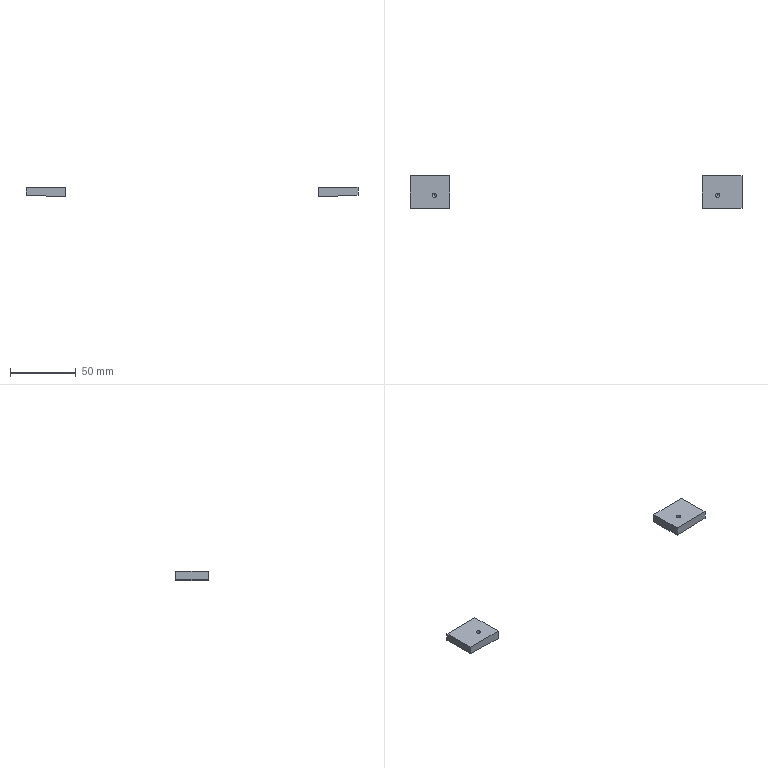Part | STEP file | 526D3-DK_AF1.stp.STEP | 2 solids | 20 faces | box 252 x 25 x 6.851 mm | volume 9576 mm3 | plane 10 | cylinder 6 | cone 4 | commonest cylinder face diameters 3.3 x4 7830 x2
STEP:
#1=CARTESIAN_POINT('',(-107.5,-0.85,-5.));
#2=VERTEX_POINT('',#1);
#3=CARTESIAN_POINT('',(-107.5,-0.85,0.));
#4=VERTEX_POINT('',#3);
#5=CARTESIAN_POINT('',(-107.5,-0.85,-5.));
#6=DIRECTION('',(0.,0.,1.));
#7=VECTOR('',#6,1000.);
#8=LINE('',#5,#7);
#9=EDGE_CURVE('',#2,#4,#8,.T.);
#10=ORIENTED_EDGE('',*,*,#9,.F.);
#11=CARTESIAN_POINT('',(-107.5,-4.15,-5.));
#12=VERTEX_POINT('',#11);
#13=CARTESIAN_POINT('',(-107.5,-2.5,-5.));
#14=DIRECTION('',(0.,0.,-1.));
#15=DIRECTION('',(0.,1.,0.));
#16=AXIS2_PLACEMENT_3D('',#13,#14,#15);
#17=CIRCLE('',#16,1.65);
#18=EDGE_CURVE('',#2,#12,#17,.T.);
#19=ORIENTED_EDGE('',*,*,#18,.T.);
#20=CARTESIAN_POINT('',(-107.5,-4.15,0.));
#21=VERTEX_POINT('',#20);
#22=CARTESIAN_POINT('',(-107.5,-4.15,-5.));
#23=DIRECTION('',(0.,0.,1.));
#24=VECTOR('',#23,1000.);
#25=LINE('',#22,#24);
#26=EDGE_CURVE('',#12,#21,#25,.T.);
#27=ORIENTED_EDGE('',*,*,#26,.T.);
#28=CARTESIAN_POINT('',(-107.5,-2.5,0.));
#29=DIRECTION('',(0.,0.,1.));
#30=DIRECTION('',(0.,-1.,0.));
#31=AXIS2_PLACEMENT_3D('',#28,#29,#30);
#32=CIRCLE('',#31,1.65);
#33=EDGE_CURVE('',#21,#4,#32,.T.);
#34=ORIENTED_EDGE('',*,*,#33,.T.);
#35=EDGE_LOOP('',(#10,#19,#27,#34));
#36=FACE_OUTER_BOUND('',#35,.T.);
#37=CARTESIAN_POINT('',(-107.5,-2.5,-6.291));
#38=DIRECTION('',(0.,0.,1.));
#39=DIRECTION('',(0.,1.,0.));
#40=AXIS2_PLACEMENT_3D('',#37,#38,#39);
#41=CYLINDRICAL_SURFACE('',#40,1.65);
#42=ADVANCED_FACE('',(#36),#41,.F.);
#43=ORIENTED_EDGE('',*,*,#33,.F.);
#44=CARTESIAN_POINT('',(-107.5,-2.5,0.));
#45=DIRECTION('',(0.,0.,1.));
#46=DIRECTION('',(0.,1.,0.));
#47=AXIS2_PLACEMENT_3D('',#44,#45,#46);
#48=CIRCLE('',#47,1.65);
#49=EDGE_CURVE('',#4,#21,#48,.T.);
#50=ORIENTED_EDGE('',*,*,#49,.F.);
#51=EDGE_LOOP('',(#43,#50));
#52=FACE_BOUND('',#51,.T.);
#53=CARTESIAN_POINT('',(-126.,12.5,0.));
#54=VERTEX_POINT('',#53);
#55=CARTESIAN_POINT('',(-96.,12.5,0.));
#56=VERTEX_POINT('',#55);
#57=CARTESIAN_POINT('',(-126.,12.5,0.));
#58=DIRECTION('',(1.,0.,0.));
#59=VECTOR('',#58,1000.);
#60=LINE('',#57,#59);
#61=EDGE_CURVE('',#54,#56,#60,.T.);
#62=ORIENTED_EDGE('',*,*,#61,.F.);
#63=CARTESIAN_POINT('',(-126.,-12.5,0.));
#64=VERTEX_POINT('',#63);
#65=CARTESIAN_POINT('',(-126.,-12.5,0.));
#66=DIRECTION('',(0.,1.,0.));
#67=VECTOR('',#66,1000.);
#68=LINE('',#65,#67);
#69=EDGE_CURVE('',#64,#54,#68,.T.);
#70=ORIENTED_EDGE('',*,*,#69,.F.);
#71=CARTESIAN_POINT('',(-96.,-12.5,0.));
#72=VERTEX_POINT('',#71);
#73=CARTESIAN_POINT('',(-126.,-12.5,0.));
#74=DIRECTION('',(1.,0.,0.));
#75=VECTOR('',#74,1000.);
#76=LINE('',#73,#75);
#77=EDGE_CURVE('',#64,#72,#76,.T.);
#78=ORIENTED_EDGE('',*,*,#77,.T.);
#79=CARTESIAN_POINT('',(-96.,-12.5,0.));
#80=DIRECTION('',(0.,1.,0.));
#81=VECTOR('',#80,1000.);
#82=LINE('',#79,#81);
#83=EDGE_CURVE('',#72,#56,#82,.T.);
#84=ORIENTED_EDGE('',*,*,#83,.T.);
#85=EDGE_LOOP('',(#62,#70,#78,#84));
#86=FACE_OUTER_BOUND('',#85,.T.);
#87=CARTESIAN_POINT('',(-126.,-12.5,0.));
#88=DIRECTION('',(0.,0.,1.));
#89=DIRECTION('',(1.,0.,0.));
#90=AXIS2_PLACEMENT_3D('',#87,#88,#89);
#91=PLANE('',#90);
#92=ADVANCED_FACE('',(#52,#86),#91,.T.);
#93=CARTESIAN_POINT('',(-96.,-12.5,-6.851));
#94=VERTEX_POINT('',#93);
#95=CARTESIAN_POINT('',(-96.,12.5,-6.851));
#96=VERTEX_POINT('',#95);
#97=CARTESIAN_POINT('',(-96.,-12.5,-6.851));
#98=DIRECTION('',(0.,1.,0.));
#99=VECTOR('',#98,1000.);
#100=LINE('',#97,#99);
#101=EDGE_CURVE('',#94,#96,#100,.T.);
#102=ORIENTED_EDGE('',*,*,#101,.T.);
#103=CARTESIAN_POINT('',(-96.,12.5,0.));
#104=DIRECTION('',(0.,0.,-1.));
#105=VECTOR('',#104,1000.);
#106=LINE('',#103,#105);
#107=EDGE_CURVE('',#56,#96,#106,.T.);
#108=ORIENTED_EDGE('',*,*,#107,.F.);
#109=ORIENTED_EDGE('',*,*,#83,.F.);
#110=CARTESIAN_POINT('',(-96.,-12.5,0.));
#111=DIRECTION('',(0.,0.,-1.));
#112=VECTOR('',#111,1000.);
#113=LINE('',#110,#112);
#114=EDGE_CURVE('',#72,#94,#113,.T.);
#115=ORIENTED_EDGE('',*,*,#114,.T.);
#116=EDGE_LOOP('',(#102,#108,#109,#115));
#117=FACE_OUTER_BOUND('',#116,.T.);
#118=CARTESIAN_POINT('',(-96.,12.5,-71.747));
#119=DIRECTION('',(-1.,0.,0.));
#120=DIRECTION('',(0.,0.,1.));
#121=AXIS2_PLACEMENT_3D('',#118,#119,#120);
#122=PLANE('',#121);
#123=ADVANCED_FACE('',(#117),#122,.F.);
#124=ORIENTED_EDGE('',*,*,#77,.F.);
#125=CARTESIAN_POINT('',(-126.,-12.5,-6.));
#126=VERTEX_POINT('',#125);
#127=CARTESIAN_POINT('',(-126.,-12.5,-6.));
#128=DIRECTION('',(0.,0.,1.));
#129=VECTOR('',#128,1000.);
#130=LINE('',#127,#129);
#131=EDGE_CURVE('',#126,#64,#130,.T.);
#132=ORIENTED_EDGE('',*,*,#131,.F.);
#133=CARTESIAN_POINT('',(0.,-12.5,3906.772));
#134=DIRECTION('',(0.,1.,0.));
#135=DIRECTION('',(-0.02452,0.,-0.9997));
#136=AXIS2_PLACEMENT_3D('',#133,#134,#135);
#137=CIRCLE('',#136,3914.8);
#138=EDGE_CURVE('',#94,#126,#137,.T.);
#139=ORIENTED_EDGE('',*,*,#138,.F.);
#140=ORIENTED_EDGE('',*,*,#114,.F.);
#141=EDGE_LOOP('',(#124,#132,#139,#140));
#142=FACE_OUTER_BOUND('',#141,.T.);
#143=CARTESIAN_POINT('',(0.,-12.5,0.));
#144=DIRECTION('',(0.,1.,0.));
#145=DIRECTION('',(1.,0.,0.));
#146=AXIS2_PLACEMENT_3D('',#143,#144,#145);
#147=PLANE('',#146);
#148=ADVANCED_FACE('',(#142),#147,.F.);
#149=ORIENTED_EDGE('',*,*,#138,.T.);
#150=CARTESIAN_POINT('',(-126.,12.5,-6.));
#151=VERTEX_POINT('',#150);
#152=CARTESIAN_POINT('',(-126.,-12.5,-6.));
#153=DIRECTION('',(0.,1.,0.));
#154=VECTOR('',#153,1000.);
#155=LINE('',#152,#154);
#156=EDGE_CURVE('',#126,#151,#155,.T.);
#157=ORIENTED_EDGE('',*,*,#156,.T.);
#158=CARTESIAN_POINT('',(0.,12.5,3906.772));
#159=DIRECTION('',(0.,1.,0.));
#160=DIRECTION('',(-0.02452,0.,-0.9997));
#161=AXIS2_PLACEMENT_3D('',#158,#159,#160);
#162=CIRCLE('',#161,3914.8);
#163=EDGE_CURVE('',#96,#151,#162,.T.);
#164=ORIENTED_EDGE('',*,*,#163,.F.);
#165=ORIENTED_EDGE('',*,*,#101,.F.);
#166=EDGE_LOOP('',(#149,#157,#164,#165));
#167=FACE_OUTER_BOUND('',#166,.T.);
#168=CARTESIAN_POINT('',(0.,-12.5,3906.772));
#169=DIRECTION('',(0.,1.,0.));
#170=DIRECTION('',(1.,0.,0.));
#171=AXIS2_PLACEMENT_3D('',#168,#169,#170);
#172=CYLINDRICAL_SURFACE('',#171,3914.8);
#173=ADVANCED_FACE('',(#167),#172,.T.);
#174=ORIENTED_EDGE('',*,*,#163,.T.);
#175=CARTESIAN_POINT('',(-126.,12.5,-6.));
#176=DIRECTION('',(0.,0.,1.));
#177=VECTOR('',#176,1000.);
#178=LINE('',#175,#177);
#179=EDGE_CURVE('',#151,#54,#178,.T.);
#180=ORIENTED_EDGE('',*,*,#179,.T.);
#181=ORIENTED_EDGE('',*,*,#61,.T.);
#182=ORIENTED_EDGE('',*,*,#107,.T.);
#183=EDGE_LOOP('',(#174,#180,#181,#182));
#184=FACE_OUTER_BOUND('',#183,.T.);
#185=CARTESIAN_POINT('',(0.,12.5,0.));
#186=DIRECTION('',(0.,1.,0.));
#187=DIRECTION('',(1.,0.,0.));
#188=AXIS2_PLACEMENT_3D('',#185,#186,#187);
#189=PLANE('',#188);
#190=ADVANCED_FACE('',(#184),#189,.T.);
#191=ORIENTED_EDGE('',*,*,#69,.T.);
#192=ORIENTED_EDGE('',*,*,#179,.F.);
#193=ORIENTED_EDGE('',*,*,#156,.F.);
#194=ORIENTED_EDGE('',*,*,#131,.T.);
#195=EDGE_LOOP('',(#191,#192,#193,#194));
#196=FACE_OUTER_BOUND('',#195,.T.);
#197=CARTESIAN_POINT('',(-126.,-12.5,-6.));
#198=DIRECTION('',(-1.,0.,0.));
#199=DIRECTION('',(0.,0.,1.));
#200=AXIS2_PLACEMENT_3D('',#197,#198,#199);
#201=PLANE('',#200);
#202=ADVANCED_FACE('',(#196),#201,.T.);
#203=ORIENTED_EDGE('',*,*,#26,.F.);
#204=CARTESIAN_POINT('',(-107.5,-2.5,-5.));
#205=DIRECTION('',(0.,0.,1.));
#206=DIRECTION('',(0.,1.,0.));
#207=AXIS2_PLACEMENT_3D('',#204,#205,#206);
#208=CIRCLE('',#207,1.65);
#209=EDGE_CURVE('',#2,#12,#208,.T.);
#210=ORIENTED_EDGE('',*,*,#209,.F.);
#211=ORIENTED_EDGE('',*,*,#9,.T.);
#212=ORIENTED_EDGE('',*,*,#49,.T.);
#213=EDGE_LOOP('',(#203,#210,#211,#212));
#214=FACE_OUTER_BOUND('',#213,.T.);
#215=CARTESIAN_POINT('',(-107.5,-2.5,-6.291));
#216=DIRECTION('',(0.,0.,1.));
#217=DIRECTION('',(0.,1.,0.));
#218=AXIS2_PLACEMENT_3D('',#215,#216,#217);
#219=CYLINDRICAL_SURFACE('',#218,1.65);
#220=ADVANCED_FACE('',(#214),#219,.F.);
#221=ORIENTED_EDGE('',*,*,#209,.T.);
#222=CARTESIAN_POINT('',(-107.5,-2.5,-5.991));
#223=VERTEX_POINT('',#222);
#224=CARTESIAN_POINT('',(-107.5,-2.5,-5.991));
#225=DIRECTION('',(0.,-0.8572,0.515));
#226=VECTOR('',#225,1000.);
#227=LINE('',#224,#226);
#228=EDGE_CURVE('',#223,#12,#227,.T.);
#229=ORIENTED_EDGE('',*,*,#228,.F.);
#230=CARTESIAN_POINT('',(-107.5,-2.5,-5.991));
#231=DIRECTION('',(0.,0.8572,0.515));
#232=VECTOR('',#231,1000.);
#233=LINE('',#230,#232);
#234=EDGE_CURVE('',#223,#2,#233,.T.);
#235=ORIENTED_EDGE('',*,*,#234,.T.);
#236=EDGE_LOOP('',(#221,#229,#235));
#237=FACE_OUTER_BOUND('',#236,.T.);
#238=CARTESIAN_POINT('',(-107.5,-2.5,-5.413));
#239=DIRECTION('',(0.,0.,1.));
#240=DIRECTION('',(0.,1.,0.));
#241=AXIS2_PLACEMENT_3D('',#238,#239,#240);
#242=CONICAL_SURFACE('',#241,0.9632,1.03);
#243=ADVANCED_FACE('',(#237),#242,.F.);
#244=ORIENTED_EDGE('',*,*,#228,.T.);
#245=ORIENTED_EDGE('',*,*,#18,.F.);
#246=ORIENTED_EDGE('',*,*,#234,.F.);
#247=EDGE_LOOP('',(#244,#245,#246));
#248=FACE_OUTER_BOUND('',#247,.T.);
#249=CARTESIAN_POINT('',(-107.5,-2.5,-5.413));
#250=DIRECTION('',(0.,0.,1.));
#251=DIRECTION('',(0.,1.,0.));
#252=AXIS2_PLACEMENT_3D('',#249,#250,#251);
#253=CONICAL_SURFACE('',#252,0.9632,1.03);
#254=ADVANCED_FACE('',(#248),#253,.F.);
#255=CLOSED_SHELL('',(#42,#92,#123,#148,#173,#190,#202,#220,#243,#254));
#256=MANIFOLD_SOLID_BREP('',#255);
#257=CARTESIAN_POINT('',(107.5,-0.85,-5.));
#258=VERTEX_POINT('',#257);
#259=CARTESIAN_POINT('',(107.5,-0.85,0.));
#260=VERTEX_POINT('',#259);
#261=CARTESIAN_POINT('',(107.5,-0.85,-5.));
#262=DIRECTION('',(0.,0.,1.));
#263=VECTOR('',#262,1000.);
#264=LINE('',#261,#263);
#265=EDGE_CURVE('',#258,#260,#264,.T.);
#266=ORIENTED_EDGE('',*,*,#265,.F.);
#267=CARTESIAN_POINT('',(107.5,-4.15,-5.));
#268=VERTEX_POINT('',#267);
#269=CARTESIAN_POINT('',(107.5,-2.5,-5.));
#270=DIRECTION('',(0.,0.,-1.));
#271=DIRECTION('',(0.,1.,0.));
#272=AXIS2_PLACEMENT_3D('',#269,#270,#271);
#273=CIRCLE('',#272,1.65);
#274=EDGE_CURVE('',#258,#268,#273,.T.);
#275=ORIENTED_EDGE('',*,*,#274,.T.);
#276=CARTESIAN_POINT('',(107.5,-4.15,0.));
#277=VERTEX_POINT('',#276);
#278=CARTESIAN_POINT('',(107.5,-4.15,-5.));
#279=DIRECTION('',(0.,0.,1.));
#280=VECTOR('',#279,1000.);
#281=LINE('',#278,#280);
#282=EDGE_CURVE('',#268,#277,#281,.T.);
#283=ORIENTED_EDGE('',*,*,#282,.T.);
#284=CARTESIAN_POINT('',(107.5,-2.5,0.));
#285=DIRECTION('',(0.,0.,1.));
#286=DIRECTION('',(0.,-1.,0.));
#287=AXIS2_PLACEMENT_3D('',#284,#285,#286);
#288=CIRCLE('',#287,1.65);
#289=EDGE_CURVE('',#277,#260,#288,.T.);
#290=ORIENTED_EDGE('',*,*,#289,.T.);
#291=EDGE_LOOP('',(#266,#275,#283,#290));
#292=FACE_OUTER_BOUND('',#291,.T.);
#293=CARTESIAN_POINT('',(107.5,-2.5,-6.291));
#294=DIRECTION('',(0.,0.,1.));
#295=DIRECTION('',(0.,1.,0.));
#296=AXIS2_PLACEMENT_3D('',#293,#294,#295);
#297=CYLINDRICAL_SURFACE('',#296,1.65);
#298=ADVANCED_FACE('',(#292),#297,.F.);
#299=ORIENTED_EDGE('',*,*,#289,.F.);
#300=CARTESIAN_POINT('',(107.5,-2.5,0.));
#301=DIRECTION('',(0.,0.,1.));
#302=DIRECTION('',(0.,1.,0.));
#303=AXIS2_PLACEMENT_3D('',#300,#301,#302);
#304=CIRCLE('',#303,1.65);
#305=EDGE_CURVE('',#260,#277,#304,.T.);
#306=ORIENTED_EDGE('',*,*,#305,.F.);
#307=EDGE_LOOP('',(#299,#306));
#308=FACE_BOUND('',#307,.T.);
#309=CARTESIAN_POINT('',(96.,-12.5,0.));
#310=VERTEX_POINT('',#309);
#311=CARTESIAN_POINT('',(126.,-12.5,0.));
#312=VERTEX_POINT('',#311);
#313=CARTESIAN_POINT('',(96.,-12.5,0.));
#314=DIRECTION('',(1.,0.,0.));
#315=VECTOR('',#314,1000.);
#316=LINE('',#313,#315);
#317=EDGE_CURVE('',#310,#312,#316,.T.);
#318=ORIENTED_EDGE('',*,*,#317,.T.);
#319=CARTESIAN_POINT('',(126.,12.5,0.));
#320=VERTEX_POINT('',#319);
#321=CARTESIAN_POINT('',(126.,-12.5,0.));
#322=DIRECTION('',(0.,1.,0.));
#323=VECTOR('',#322,1000.);
#324=LINE('',#321,#323);
#325=EDGE_CURVE('',#312,#320,#324,.T.);
#326=ORIENTED_EDGE('',*,*,#325,.T.);
#327=CARTESIAN_POINT('',(96.,12.5,0.));
#328=VERTEX_POINT('',#327);
#329=CARTESIAN_POINT('',(96.,12.5,0.));
#330=DIRECTION('',(1.,0.,0.));
#331=VECTOR('',#330,1000.);
#332=LINE('',#329,#331);
#333=EDGE_CURVE('',#328,#320,#332,.T.);
#334=ORIENTED_EDGE('',*,*,#333,.F.);
#335=CARTESIAN_POINT('',(96.,-12.5,0.));
#336=DIRECTION('',(0.,1.,0.));
#337=VECTOR('',#336,1000.);
#338=LINE('',#335,#337);
#339=EDGE_CURVE('',#310,#328,#338,.T.);
#340=ORIENTED_EDGE('',*,*,#339,.F.);
#341=EDGE_LOOP('',(#318,#326,#334,#340));
#342=FACE_OUTER_BOUND('',#341,.T.);
#343=CARTESIAN_POINT('',(-126.,-12.5,0.));
#344=DIRECTION('',(0.,0.,1.));
#345=DIRECTION('',(1.,0.,0.));
#346=AXIS2_PLACEMENT_3D('',#343,#344,#345);
#347=PLANE('',#346);
#348=ADVANCED_FACE('',(#308,#342),#347,.T.);
#349=ORIENTED_EDGE('',*,*,#339,.T.);
#350=CARTESIAN_POINT('',(96.,12.5,-6.851));
#351=VERTEX_POINT('',#350);
#352=CARTESIAN_POINT('',(96.,12.5,0.));
#353=DIRECTION('',(0.,0.,-1.));
#354=VECTOR('',#353,1000.);
#355=LINE('',#352,#354);
#356=EDGE_CURVE('',#328,#351,#355,.T.);
#357=ORIENTED_EDGE('',*,*,#356,.T.);
#358=CARTESIAN_POINT('',(96.,-12.5,-6.851));
#359=VERTEX_POINT('',#358);
#360=CARTESIAN_POINT('',(96.,-12.5,-6.851));
#361=DIRECTION('',(0.,1.,0.));
#362=VECTOR('',#361,1000.);
#363=LINE('',#360,#362);
#364=EDGE_CURVE('',#359,#351,#363,.T.);
#365=ORIENTED_EDGE('',*,*,#364,.F.);
#366=CARTESIAN_POINT('',(96.,-12.5,0.));
#367=DIRECTION('',(0.,0.,-1.));
#368=VECTOR('',#367,1000.);
#369=LINE('',#366,#368);
#370=EDGE_CURVE('',#310,#359,#369,.T.);
#371=ORIENTED_EDGE('',*,*,#370,.F.);
#372=EDGE_LOOP('',(#349,#357,#365,#371));
#373=FACE_OUTER_BOUND('',#372,.T.);
#374=CARTESIAN_POINT('',(96.,12.5,18.253));
#375=DIRECTION('',(1.,0.,0.));
#376=DIRECTION('',(0.,1.,0.));
#377=AXIS2_PLACEMENT_3D('',#374,#375,#376);
#378=PLANE('',#377);
#379=ADVANCED_FACE('',(#373),#378,.F.);
#380=CARTESIAN_POINT('',(126.,-12.5,-6.));
#381=VERTEX_POINT('',#380);
#382=CARTESIAN_POINT('',(0.,-12.5,3906.772));
#383=DIRECTION('',(0.,1.,0.));
#384=DIRECTION('',(0.03219,0.,-0.9995));
#385=AXIS2_PLACEMENT_3D('',#382,#383,#384);
#386=CIRCLE('',#385,3914.8);
#387=EDGE_CURVE('',#381,#359,#386,.T.);
#388=ORIENTED_EDGE('',*,*,#387,.F.);
#389=CARTESIAN_POINT('',(126.,-12.5,0.));
#390=DIRECTION('',(0.,0.,-1.));
#391=VECTOR('',#390,1000.);
#392=LINE('',#389,#391);
#393=EDGE_CURVE('',#312,#381,#392,.T.);
#394=ORIENTED_EDGE('',*,*,#393,.F.);
#395=ORIENTED_EDGE('',*,*,#317,.F.);
#396=ORIENTED_EDGE('',*,*,#370,.T.);
#397=EDGE_LOOP('',(#388,#394,#395,#396));
#398=FACE_OUTER_BOUND('',#397,.T.);
#399=CARTESIAN_POINT('',(0.,-12.5,0.));
#400=DIRECTION('',(0.,1.,0.));
#401=DIRECTION('',(1.,0.,0.));
#402=AXIS2_PLACEMENT_3D('',#399,#400,#401);
#403=PLANE('',#402);
#404=ADVANCED_FACE('',(#398),#403,.F.);
#405=CARTESIAN_POINT('',(126.,12.5,-6.));
#406=VERTEX_POINT('',#405);
#407=CARTESIAN_POINT('',(126.,-12.5,-6.));
#408=DIRECTION('',(0.,1.,0.));
#409=VECTOR('',#408,1000.);
#410=LINE('',#407,#409);
#411=EDGE_CURVE('',#381,#406,#410,.T.);
#412=ORIENTED_EDGE('',*,*,#411,.T.);
#413=CARTESIAN_POINT('',(126.,12.5,0.));
#414=DIRECTION('',(0.,0.,-1.));
#415=VECTOR('',#414,1000.);
#416=LINE('',#413,#415);
#417=EDGE_CURVE('',#320,#406,#416,.T.);
#418=ORIENTED_EDGE('',*,*,#417,.F.);
#419=ORIENTED_EDGE('',*,*,#325,.F.);
#420=ORIENTED_EDGE('',*,*,#393,.T.);
#421=EDGE_LOOP('',(#412,#418,#419,#420));
#422=FACE_OUTER_BOUND('',#421,.T.);
#423=CARTESIAN_POINT('',(126.,-12.5,0.));
#424=DIRECTION('',(1.,0.,0.));
#425=DIRECTION('',(0.,1.,0.));
#426=AXIS2_PLACEMENT_3D('',#423,#424,#425);
#427=PLANE('',#426);
#428=ADVANCED_FACE('',(#422),#427,.T.);
#429=ORIENTED_EDGE('',*,*,#333,.T.);
#430=ORIENTED_EDGE('',*,*,#417,.T.);
#431=CARTESIAN_POINT('',(0.,12.5,3906.772));
#432=DIRECTION('',(0.,1.,0.));
#433=DIRECTION('',(0.03219,0.,-0.9995));
#434=AXIS2_PLACEMENT_3D('',#431,#432,#433);
#435=CIRCLE('',#434,3914.8);
#436=EDGE_CURVE('',#406,#351,#435,.T.);
#437=ORIENTED_EDGE('',*,*,#436,.T.);
#438=ORIENTED_EDGE('',*,*,#356,.F.);
#439=EDGE_LOOP('',(#429,#430,#437,#438));
#440=FACE_OUTER_BOUND('',#439,.T.);
#441=CARTESIAN_POINT('',(0.,12.5,0.));
#442=DIRECTION('',(0.,1.,0.));
#443=DIRECTION('',(1.,0.,0.));
#444=AXIS2_PLACEMENT_3D('',#441,#442,#443);
#445=PLANE('',#444);
#446=ADVANCED_FACE('',(#440),#445,.T.);
#447=ORIENTED_EDGE('',*,*,#436,.F.);
#448=ORIENTED_EDGE('',*,*,#411,.F.);
#449=ORIENTED_EDGE('',*,*,#387,.T.);
#450=ORIENTED_EDGE('',*,*,#364,.T.);
#451=EDGE_LOOP('',(#447,#448,#449,#450));
#452=FACE_OUTER_BOUND('',#451,.T.);
#453=CARTESIAN_POINT('',(0.,-12.5,3906.772));
#454=DIRECTION('',(0.,1.,0.));
#455=DIRECTION('',(1.,0.,0.));
#456=AXIS2_PLACEMENT_3D('',#453,#454,#455);
#457=CYLINDRICAL_SURFACE('',#456,3914.8);
#458=ADVANCED_FACE('',(#452),#457,.T.);
#459=ORIENTED_EDGE('',*,*,#282,.F.);
#460=CARTESIAN_POINT('',(107.5,-2.5,-5.));
#461=DIRECTION('',(0.,0.,1.));
#462=DIRECTION('',(0.,1.,0.));
#463=AXIS2_PLACEMENT_3D('',#460,#461,#462);
#464=CIRCLE('',#463,1.65);
#465=EDGE_CURVE('',#258,#268,#464,.T.);
#466=ORIENTED_EDGE('',*,*,#465,.F.);
#467=ORIENTED_EDGE('',*,*,#265,.T.);
#468=ORIENTED_EDGE('',*,*,#305,.T.);
#469=EDGE_LOOP('',(#459,#466,#467,#468));
#470=FACE_OUTER_BOUND('',#469,.T.);
#471=CARTESIAN_POINT('',(107.5,-2.5,-6.291));
#472=DIRECTION('',(0.,0.,1.));
#473=DIRECTION('',(0.,1.,0.));
#474=AXIS2_PLACEMENT_3D('',#471,#472,#473);
#475=CYLINDRICAL_SURFACE('',#474,1.65);
#476=ADVANCED_FACE('',(#470),#475,.F.);
#477=ORIENTED_EDGE('',*,*,#465,.T.);
#478=CARTESIAN_POINT('',(107.5,-2.5,-5.991));
#479=VERTEX_POINT('',#478);
#480=CARTESIAN_POINT('',(107.5,-2.5,-5.991));
#481=DIRECTION('',(0.,-0.8572,0.515));
#482=VECTOR('',#481,1000.);
#483=LINE('',#480,#482);
#484=EDGE_CURVE('',#479,#268,#483,.T.);
#485=ORIENTED_EDGE('',*,*,#484,.F.);
#486=CARTESIAN_POINT('',(107.5,-2.5,-5.991));
#487=DIRECTION('',(0.,0.8572,0.515));
#488=VECTOR('',#487,1000.);
#489=LINE('',#486,#488);
#490=EDGE_CURVE('',#479,#258,#489,.T.);
#491=ORIENTED_EDGE('',*,*,#490,.T.);
#492=EDGE_LOOP('',(#477,#485,#491));
#493=FACE_OUTER_BOUND('',#492,.T.);
#494=CARTESIAN_POINT('',(107.5,-2.5,-5.413));
#495=DIRECTION('',(0.,0.,1.));
#496=DIRECTION('',(0.,1.,0.));
#497=AXIS2_PLACEMENT_3D('',#494,#495,#496);
#498=CONICAL_SURFACE('',#497,0.9632,1.03);
#499=ADVANCED_FACE('',(#493),#498,.F.);
#500=ORIENTED_EDGE('',*,*,#484,.T.);
#501=ORIENTED_EDGE('',*,*,#274,.F.);
#502=ORIENTED_EDGE('',*,*,#490,.F.);
#503=EDGE_LOOP('',(#500,#501,#502));
#504=FACE_OUTER_BOUND('',#503,.T.);
#505=CARTESIAN_POINT('',(107.5,-2.5,-5.413));
#506=DIRECTION('',(0.,0.,1.));
#507=DIRECTION('',(0.,1.,0.));
#508=AXIS2_PLACEMENT_3D('',#505,#506,#507);
#509=CONICAL_SURFACE('',#508,0.9632,1.03);
#510=ADVANCED_FACE('',(#504),#509,.F.);
#511=CLOSED_SHELL('',(#298,#348,#379,#404,#428,#446,#458,#476,#499,#510));
#512=MANIFOLD_SOLID_BREP('',#511);
#513=CARTESIAN_POINT('',(0.,0.,0.));
#514=DIRECTION('',(0.,0.,1.));
#515=DIRECTION('',(1.,0.,0.));
#516=AXIS2_PLACEMENT_3D('',#513,#514,#515);
#517=(LENGTH_UNIT()NAMED_UNIT(*)SI_UNIT(.MILLI.,.METRE.));
#518=UNCERTAINTY_MEASURE_WITH_UNIT(LENGTH_MEASURE(0.00001),#517,'','');
#519=(NAMED_UNIT(*)PLANE_ANGLE_UNIT()SI_UNIT($,.RADIAN.));
#520=(NAMED_UNIT(*)SI_UNIT($,.STERADIAN.)SOLID_ANGLE_UNIT());
#521=(GEOMETRIC_REPRESENTATION_CONTEXT(3)GLOBAL_UNCERTAINTY_ASSIGNED_CONTEXT((#518))GLOBAL_UNIT_ASSIGNED_CONTEXT((#517,#519,#520))REPRESENTATION_CONTEXT('',''));
#522=ADVANCED_BREP_SHAPE_REPRESENTATION('',(#256,#512,#516),#521);